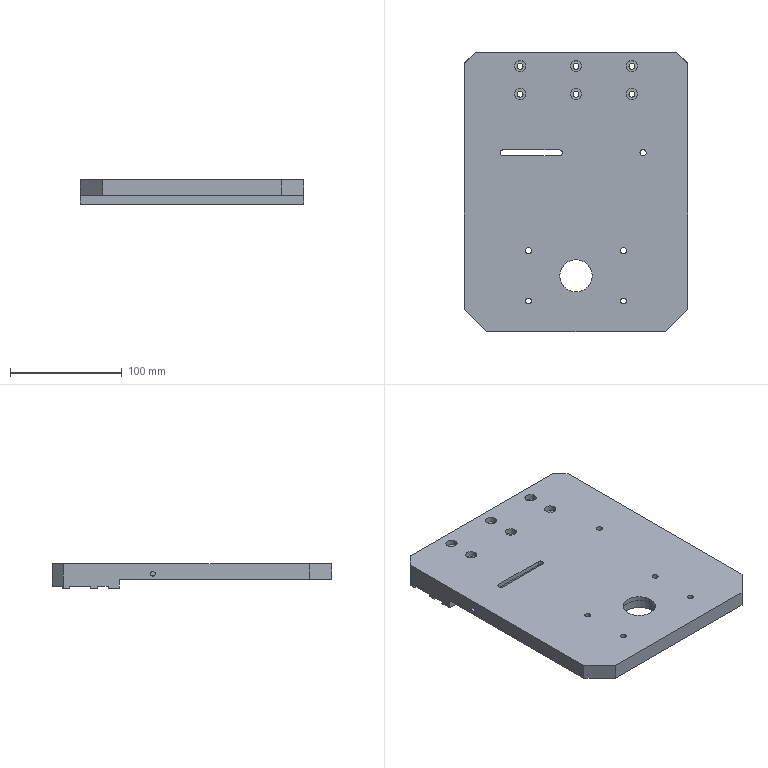Part | STEP file | CON-003 | 1 solid | 95 faces | box 200 x 250 x 22 mm | volume 741218 mm3 | cylinder 56 | plane 39 | commonest cylinder face diameters 5.3 x20 10 x20 5.5 x5 15 x5 4.2 x2 29 x2